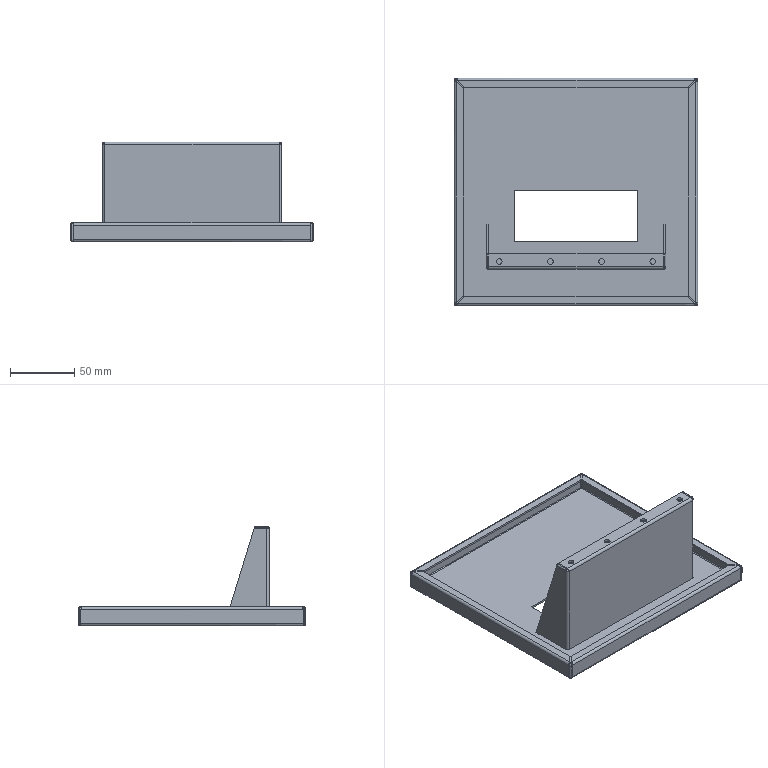Part | SolidWorks | features SMWeldBead 6, EdgeFlange 3, FlatPattern 2, HoleWzd 2, SMBaseFlange 2, SheetMetal 2, Chamfer 1, ICE 1 | 2 solids | 170 faces | box 190 x 178 x 78 mm | volume 87665 mm3 | plane 84 | cylinder 44 | spline 42 | commonest cylinder face diameters 1 x15 4 x15 4.5 x8 2 x6